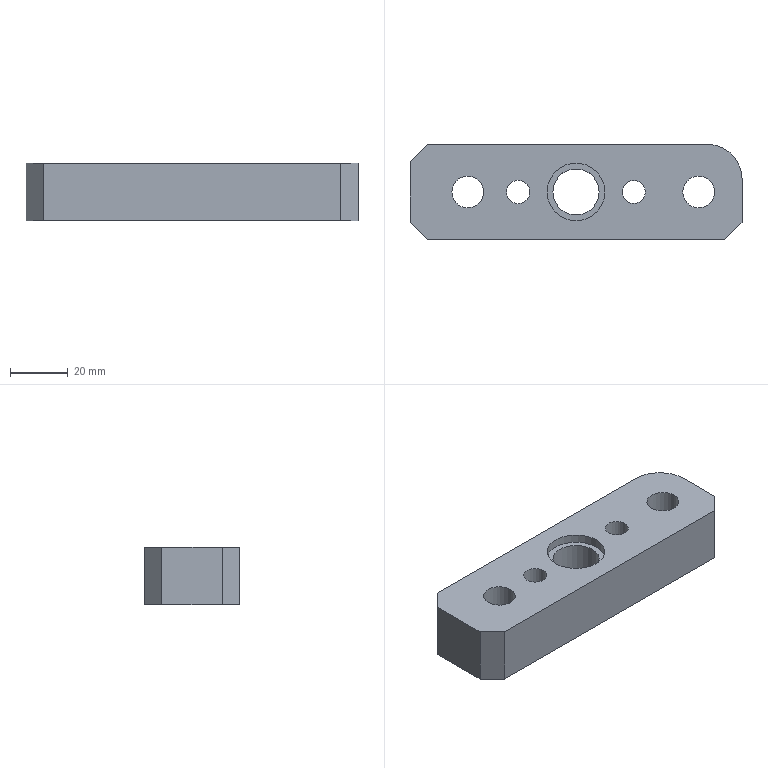Part | STEP file | 103_id3510_x_t | 1 solid | 21 faces | box 115 x 32.999 x 20 mm | volume 61100 mm3 | plane 12 | cylinder 9 | commonest cylinder face diameters 11 x2 17 x2 8 x1 8.1 x1 16 x1 20 x1
STEP:
#1=CARTESIAN_POINT('',(3521.,-0.01549,22.5));
#2=VERTEX_POINT('',#1);
#3=CARTESIAN_POINT('',(3526.5,-0.01549,22.5));
#4=DIRECTION('',(0.,0.,1.));
#5=DIRECTION('',(-1.,0.,0.));
#6=AXIS2_PLACEMENT_3D('',#3,#4,#5);
#7=CIRCLE('',#6,5.5);
#8=EDGE_CURVE('',#2,#2,#7,.T.);
#9=ORIENTED_EDGE('',*,*,#8,.F.);
#10=EDGE_LOOP('',(#9));
#11=FACE_BOUND('',#10,.T.);
#12=CARTESIAN_POINT('',(3601.,-0.01549,22.5));
#13=VERTEX_POINT('',#12);
#14=CARTESIAN_POINT('',(3606.5,-0.01549,22.5));
#15=DIRECTION('',(0.,0.,1.));
#16=DIRECTION('',(-1.,0.,0.));
#17=AXIS2_PLACEMENT_3D('',#14,#15,#16);
#18=CIRCLE('',#17,5.5);
#19=EDGE_CURVE('',#13,#13,#18,.T.);
#20=ORIENTED_EDGE('',*,*,#19,.F.);
#21=EDGE_LOOP('',(#20));
#22=FACE_BOUND('',#21,.T.);
#23=CARTESIAN_POINT('',(3554.,0.,22.5));
#24=VERTEX_POINT('',#23);
#25=CARTESIAN_POINT('',(3564.,0.,22.5));
#26=DIRECTION('',(0.,0.,-1.));
#27=DIRECTION('',(-1.,0.,0.));
#28=AXIS2_PLACEMENT_3D('',#25,#26,#27);
#29=CIRCLE('',#28,10.);
#30=EDGE_CURVE('',#24,#24,#29,.T.);
#31=ORIENTED_EDGE('',*,*,#30,.T.);
#32=EDGE_LOOP('',(#31));
#33=FACE_BOUND('',#32,.T.);
#34=CARTESIAN_POINT('',(3621.5,-10.5,22.5));
#35=VERTEX_POINT('',#34);
#36=CARTESIAN_POINT('',(3621.5,4.5,22.5));
#37=VERTEX_POINT('',#36);
#38=CARTESIAN_POINT('',(3621.5,-172.571,22.5));
#39=DIRECTION('',(0.,1.,0.));
#40=VECTOR('',#39,1.);
#41=LINE('',#38,#40);
#42=EDGE_CURVE('',#35,#37,#41,.T.);
#43=ORIENTED_EDGE('',*,*,#42,.T.);
#44=CARTESIAN_POINT('',(3609.5,16.5,22.5));
#45=VERTEX_POINT('',#44);
#46=CARTESIAN_POINT('',(3609.5,4.5,22.5));
#47=DIRECTION('',(0.,0.,1.));
#48=DIRECTION('',(1.,0.,0.));
#49=AXIS2_PLACEMENT_3D('',#46,#47,#48);
#50=CIRCLE('',#49,12.);
#51=EDGE_CURVE('',#37,#45,#50,.T.);
#52=ORIENTED_EDGE('',*,*,#51,.T.);
#53=CARTESIAN_POINT('',(3512.5,16.5,22.5));
#54=VERTEX_POINT('',#53);
#55=CARTESIAN_POINT('',(4674.5,16.5,22.5));
#56=DIRECTION('',(-1.,0.,0.));
#57=VECTOR('',#56,1.);
#58=LINE('',#55,#57);
#59=EDGE_CURVE('',#45,#54,#58,.T.);
#60=ORIENTED_EDGE('',*,*,#59,.T.);
#61=CARTESIAN_POINT('',(3506.5,10.5,22.5));
#62=VERTEX_POINT('',#61);
#63=CARTESIAN_POINT('',(3998.965,502.965,22.5));
#64=DIRECTION('',(-0.7071,-0.7071,0.));
#65=VECTOR('',#64,1.);
#66=LINE('',#63,#65);
#67=EDGE_CURVE('',#54,#62,#66,.T.);
#68=ORIENTED_EDGE('',*,*,#67,.T.);
#69=CARTESIAN_POINT('',(3506.5,-10.5,22.5));
#70=VERTEX_POINT('',#69);
#71=CARTESIAN_POINT('',(3506.5,-172.571,22.5));
#72=DIRECTION('',(0.,-1.,0.));
#73=VECTOR('',#72,1.);
#74=LINE('',#71,#73);
#75=EDGE_CURVE('',#62,#70,#74,.T.);
#76=ORIENTED_EDGE('',*,*,#75,.T.);
#77=CARTESIAN_POINT('',(3512.5,-16.5,22.5));
#78=VERTEX_POINT('',#77);
#79=CARTESIAN_POINT('',(4171.536,-675.535,22.5));
#80=DIRECTION('',(0.7071,-0.7071,0.));
#81=VECTOR('',#80,1.);
#82=LINE('',#79,#81);
#83=EDGE_CURVE('',#70,#78,#82,.T.);
#84=ORIENTED_EDGE('',*,*,#83,.T.);
#85=CARTESIAN_POINT('',(3615.5,-16.5,22.5));
#86=VERTEX_POINT('',#85);
#87=CARTESIAN_POINT('',(4674.5,-16.5,22.5));
#88=DIRECTION('',(1.,0.,0.));
#89=VECTOR('',#88,1.);
#90=LINE('',#87,#89);
#91=EDGE_CURVE('',#78,#86,#90,.T.);
#92=ORIENTED_EDGE('',*,*,#91,.T.);
#93=CARTESIAN_POINT('',(4066.965,434.965,22.5));
#94=DIRECTION('',(0.7071,0.7071,0.));
#95=VECTOR('',#94,1.);
#96=LINE('',#93,#95);
#97=EDGE_CURVE('',#86,#35,#96,.T.);
#98=ORIENTED_EDGE('',*,*,#97,.T.);
#99=EDGE_LOOP('',(#43,#52,#60,#68,#76,#84,#92,#98));
#100=FACE_BOUND('',#99,.T.);
#101=CARTESIAN_POINT('',(3588.,0.,22.5));
#102=VERTEX_POINT('',#101);
#103=CARTESIAN_POINT('',(3584.,0.,22.5));
#104=DIRECTION('',(0.,0.,1.));
#105=DIRECTION('',(1.,0.,0.));
#106=AXIS2_PLACEMENT_3D('',#103,#104,#105);
#107=CIRCLE('',#106,4.);
#108=EDGE_CURVE('',#102,#102,#107,.T.);
#109=ORIENTED_EDGE('',*,*,#108,.F.);
#110=EDGE_LOOP('',(#109));
#111=FACE_BOUND('',#110,.T.);
#112=CARTESIAN_POINT('',(3548.05,0.,22.5));
#113=VERTEX_POINT('',#112);
#114=CARTESIAN_POINT('',(3544.,0.,22.5));
#115=DIRECTION('',(0.,0.,1.));
#116=DIRECTION('',(1.,0.,0.));
#117=AXIS2_PLACEMENT_3D('',#114,#115,#116);
#118=CIRCLE('',#117,4.05);
#119=EDGE_CURVE('',#113,#113,#118,.T.);
#120=ORIENTED_EDGE('',*,*,#119,.F.);
#121=EDGE_LOOP('',(#120));
#122=FACE_BOUND('',#121,.T.);
#123=CARTESIAN_POINT('',(4674.5,-172.571,22.5));
#124=DIRECTION('',(0.,0.,1.));
#125=DIRECTION('',(-1.,0.,0.));
#126=AXIS2_PLACEMENT_3D('',#123,#124,#125);
#127=PLANE('',#126);
#128=ADVANCED_FACE('',(#11,#22,#33,#100,#111,#122),#127,.T.);
#129=ORIENTED_EDGE('',*,*,#75,.F.);
#130=CARTESIAN_POINT('',(3506.5,10.5,2.5));
#131=VERTEX_POINT('',#130);
#132=CARTESIAN_POINT('',(3506.5,10.5,17.5));
#133=DIRECTION('',(0.,0.,-1.));
#134=VECTOR('',#133,1.);
#135=LINE('',#132,#134);
#136=EDGE_CURVE('',#62,#131,#135,.T.);
#137=ORIENTED_EDGE('',*,*,#136,.T.);
#138=CARTESIAN_POINT('',(3506.5,-10.5,2.5));
#139=VERTEX_POINT('',#138);
#140=CARTESIAN_POINT('',(3506.5,-172.571,2.5));
#141=DIRECTION('',(0.,-1.,0.));
#142=VECTOR('',#141,1.);
#143=LINE('',#140,#142);
#144=EDGE_CURVE('',#131,#139,#143,.T.);
#145=ORIENTED_EDGE('',*,*,#144,.T.);
#146=CARTESIAN_POINT('',(3506.5,-10.5,17.5));
#147=DIRECTION('',(0.,0.,1.));
#148=VECTOR('',#147,1.);
#149=LINE('',#146,#148);
#150=EDGE_CURVE('',#139,#70,#149,.T.);
#151=ORIENTED_EDGE('',*,*,#150,.T.);
#152=EDGE_LOOP('',(#129,#137,#145,#151));
#153=FACE_OUTER_BOUND('',#152,.T.);
#154=CARTESIAN_POINT('',(3506.5,0.,17.5));
#155=DIRECTION('',(-1.,0.,0.));
#156=DIRECTION('',(0.,0.,-1.));
#157=AXIS2_PLACEMENT_3D('',#154,#155,#156);
#158=PLANE('',#157);
#159=ADVANCED_FACE('',(#153),#158,.T.);
#160=CARTESIAN_POINT('',(3621.5,-10.5,2.5));
#161=VERTEX_POINT('',#160);
#162=CARTESIAN_POINT('',(3621.5,4.5,2.5));
#163=VERTEX_POINT('',#162);
#164=CARTESIAN_POINT('',(3621.5,-172.571,2.5));
#165=DIRECTION('',(0.,1.,0.));
#166=VECTOR('',#165,1.);
#167=LINE('',#164,#166);
#168=EDGE_CURVE('',#161,#163,#167,.T.);
#169=ORIENTED_EDGE('',*,*,#168,.T.);
#170=CARTESIAN_POINT('',(3621.5,4.5,22.5));
#171=DIRECTION('',(0.,0.,1.));
#172=VECTOR('',#171,1.);
#173=LINE('',#170,#172);
#174=EDGE_CURVE('',#163,#37,#173,.T.);
#175=ORIENTED_EDGE('',*,*,#174,.T.);
#176=ORIENTED_EDGE('',*,*,#42,.F.);
#177=CARTESIAN_POINT('',(3621.5,-10.5,2.5));
#178=DIRECTION('',(0.,0.,-1.));
#179=VECTOR('',#178,1.);
#180=LINE('',#177,#179);
#181=EDGE_CURVE('',#35,#161,#180,.T.);
#182=ORIENTED_EDGE('',*,*,#181,.T.);
#183=EDGE_LOOP('',(#169,#175,#176,#182));
#184=FACE_OUTER_BOUND('',#183,.T.);
#185=CARTESIAN_POINT('',(3621.5,-172.571,2.5));
#186=DIRECTION('',(-1.,0.,0.));
#187=DIRECTION('',(0.,-1.,0.));
#188=AXIS2_PLACEMENT_3D('',#185,#186,#187);
#189=PLANE('',#188);
#190=ADVANCED_FACE('',(#184),#189,.F.);
#191=CARTESIAN_POINT('',(3580.,0.,2.5));
#192=VERTEX_POINT('',#191);
#193=CARTESIAN_POINT('',(3584.,0.,2.5));
#194=DIRECTION('',(0.,0.,-1.));
#195=DIRECTION('',(-1.,0.,0.));
#196=AXIS2_PLACEMENT_3D('',#193,#194,#195);
#197=CIRCLE('',#196,4.);
#198=EDGE_CURVE('',#192,#192,#197,.T.);
#199=ORIENTED_EDGE('',*,*,#198,.F.);
#200=EDGE_LOOP('',(#199));
#201=FACE_BOUND('',#200,.T.);
#202=CARTESIAN_POINT('',(3539.95,0.,2.5));
#203=VERTEX_POINT('',#202);
#204=CARTESIAN_POINT('',(3544.,0.,2.5));
#205=DIRECTION('',(0.,0.,1.));
#206=DIRECTION('',(-1.,0.,0.));
#207=AXIS2_PLACEMENT_3D('',#204,#205,#206);
#208=CIRCLE('',#207,4.05);
#209=EDGE_CURVE('',#203,#203,#208,.T.);
#210=ORIENTED_EDGE('',*,*,#209,.T.);
#211=EDGE_LOOP('',(#210));
#212=FACE_BOUND('',#211,.T.);
#213=CARTESIAN_POINT('',(3556.,0.,2.5));
#214=VERTEX_POINT('',#213);
#215=CARTESIAN_POINT('',(3564.,0.,2.5));
#216=DIRECTION('',(0.,0.,1.));
#217=DIRECTION('',(-1.,0.,0.));
#218=AXIS2_PLACEMENT_3D('',#215,#216,#217);
#219=CIRCLE('',#218,8.);
#220=EDGE_CURVE('',#214,#214,#219,.T.);
#221=ORIENTED_EDGE('',*,*,#220,.T.);
#222=EDGE_LOOP('',(#221));
#223=FACE_BOUND('',#222,.T.);
#224=CARTESIAN_POINT('',(3518.,-0.01549,2.5));
#225=VERTEX_POINT('',#224);
#226=CARTESIAN_POINT('',(3526.5,-0.01549,2.5));
#227=DIRECTION('',(0.,0.,1.));
#228=DIRECTION('',(-1.,0.,0.));
#229=AXIS2_PLACEMENT_3D('',#226,#227,#228);
#230=CIRCLE('',#229,8.5);
#231=EDGE_CURVE('',#225,#225,#230,.T.);
#232=ORIENTED_EDGE('',*,*,#231,.T.);
#233=EDGE_LOOP('',(#232));
#234=FACE_BOUND('',#233,.T.);
#235=CARTESIAN_POINT('',(3598.,-0.01549,2.5));
#236=VERTEX_POINT('',#235);
#237=CARTESIAN_POINT('',(3606.5,-0.01549,2.5));
#238=DIRECTION('',(0.,0.,1.));
#239=DIRECTION('',(-1.,0.,0.));
#240=AXIS2_PLACEMENT_3D('',#237,#238,#239);
#241=CIRCLE('',#240,8.5);
#242=EDGE_CURVE('',#236,#236,#241,.T.);
#243=ORIENTED_EDGE('',*,*,#242,.T.);
#244=EDGE_LOOP('',(#243));
#245=FACE_BOUND('',#244,.T.);
#246=CARTESIAN_POINT('',(3609.5,16.5,2.5));
#247=VERTEX_POINT('',#246);
#248=CARTESIAN_POINT('',(3512.5,16.5,2.5));
#249=VERTEX_POINT('',#248);
#250=CARTESIAN_POINT('',(3486.688,16.5,2.5));
#251=DIRECTION('',(-1.,0.,0.));
#252=VECTOR('',#251,1.);
#253=LINE('',#250,#252);
#254=EDGE_CURVE('',#247,#249,#253,.T.);
#255=ORIENTED_EDGE('',*,*,#254,.F.);
#256=CARTESIAN_POINT('',(3609.5,4.5,2.5));
#257=DIRECTION('',(0.,0.,-1.));
#258=DIRECTION('',(1.,0.,0.));
#259=AXIS2_PLACEMENT_3D('',#256,#257,#258);
#260=CIRCLE('',#259,12.);
#261=EDGE_CURVE('',#247,#163,#260,.T.);
#262=ORIENTED_EDGE('',*,*,#261,.T.);
#263=ORIENTED_EDGE('',*,*,#168,.F.);
#264=CARTESIAN_POINT('',(3615.5,-16.5,2.5));
#265=VERTEX_POINT('',#264);
#266=CARTESIAN_POINT('',(3621.5,-10.5,2.5));
#267=DIRECTION('',(-0.7071,-0.7071,0.));
#268=VECTOR('',#267,1.);
#269=LINE('',#266,#268);
#270=EDGE_CURVE('',#161,#265,#269,.T.);
#271=ORIENTED_EDGE('',*,*,#270,.T.);
#272=CARTESIAN_POINT('',(3512.5,-16.5,2.5));
#273=VERTEX_POINT('',#272);
#274=CARTESIAN_POINT('',(3486.688,-16.5,2.5));
#275=DIRECTION('',(1.,0.,0.));
#276=VECTOR('',#275,1.);
#277=LINE('',#274,#276);
#278=EDGE_CURVE('',#273,#265,#277,.T.);
#279=ORIENTED_EDGE('',*,*,#278,.F.);
#280=CARTESIAN_POINT('',(3512.5,-16.5,2.5));
#281=DIRECTION('',(-0.7071,0.7071,0.));
#282=VECTOR('',#281,1.);
#283=LINE('',#280,#282);
#284=EDGE_CURVE('',#273,#139,#283,.T.);
#285=ORIENTED_EDGE('',*,*,#284,.T.);
#286=ORIENTED_EDGE('',*,*,#144,.F.);
#287=CARTESIAN_POINT('',(3512.5,16.5,2.5));
#288=DIRECTION('',(0.7071,0.7071,0.));
#289=VECTOR('',#288,1.);
#290=LINE('',#287,#289);
#291=EDGE_CURVE('',#131,#249,#290,.T.);
#292=ORIENTED_EDGE('',*,*,#291,.T.);
#293=EDGE_LOOP('',(#255,#262,#263,#271,#279,#285,#286,#292));
#294=FACE_BOUND('',#293,.T.);
#295=CARTESIAN_POINT('',(4674.5,-172.571,2.5));
#296=DIRECTION('',(0.,0.,1.));
#297=DIRECTION('',(-1.,0.,0.));
#298=AXIS2_PLACEMENT_3D('',#295,#296,#297);
#299=PLANE('',#298);
#300=ADVANCED_FACE('',(#201,#212,#223,#234,#245,#294),#299,.F.);
#301=CARTESIAN_POINT('',(3598.,-0.01549,13.5));
#302=VERTEX_POINT('',#301);
#303=CARTESIAN_POINT('',(3606.5,-0.01549,13.5));
#304=DIRECTION('',(0.,0.,-1.));
#305=DIRECTION('',(-1.,0.,0.));
#306=AXIS2_PLACEMENT_3D('',#303,#304,#305);
#307=CIRCLE('',#306,8.5);
#308=EDGE_CURVE('',#302,#302,#307,.T.);
#309=ORIENTED_EDGE('',*,*,#308,.F.);
#310=EDGE_LOOP('',(#309));
#311=FACE_BOUND('',#310,.T.);
#312=ORIENTED_EDGE('',*,*,#242,.F.);
#313=EDGE_LOOP('',(#312));
#314=FACE_BOUND('',#313,.T.);
#315=CARTESIAN_POINT('',(3606.5,-0.01549,-35.5));
#316=DIRECTION('',(0.,0.,1.));
#317=DIRECTION('',(-1.,0.,0.));
#318=AXIS2_PLACEMENT_3D('',#315,#316,#317);
#319=CYLINDRICAL_SURFACE('',#318,8.5);
#320=ADVANCED_FACE('',(#311,#314),#319,.F.);
#321=CARTESIAN_POINT('',(3601.,-0.01549,13.5));
#322=VERTEX_POINT('',#321);
#323=CARTESIAN_POINT('',(3606.5,-0.01549,13.5));
#324=DIRECTION('',(0.,0.,-1.));
#325=DIRECTION('',(-1.,0.,0.));
#326=AXIS2_PLACEMENT_3D('',#323,#324,#325);
#327=CIRCLE('',#326,5.5);
#328=EDGE_CURVE('',#322,#322,#327,.T.);
#329=ORIENTED_EDGE('',*,*,#328,.F.);
#330=EDGE_LOOP('',(#329));
#331=FACE_BOUND('',#330,.T.);
#332=ORIENTED_EDGE('',*,*,#308,.T.);
#333=EDGE_LOOP('',(#332));
#334=FACE_BOUND('',#333,.T.);
#335=CARTESIAN_POINT('',(3606.5,-0.01549,13.5));
#336=DIRECTION('',(0.,0.,1.));
#337=DIRECTION('',(-1.,0.,0.));
#338=AXIS2_PLACEMENT_3D('',#335,#336,#337);
#339=PLANE('',#338);
#340=ADVANCED_FACE('',(#331,#334),#339,.F.);
#341=ORIENTED_EDGE('',*,*,#19,.T.);
#342=EDGE_LOOP('',(#341));
#343=FACE_BOUND('',#342,.T.);
#344=ORIENTED_EDGE('',*,*,#328,.T.);
#345=EDGE_LOOP('',(#344));
#346=FACE_BOUND('',#345,.T.);
#347=CARTESIAN_POINT('',(3606.5,-0.01549,14.5));
#348=DIRECTION('',(0.,0.,1.));
#349=DIRECTION('',(-1.,0.,0.));
#350=AXIS2_PLACEMENT_3D('',#347,#348,#349);
#351=CYLINDRICAL_SURFACE('',#350,5.5);
#352=ADVANCED_FACE('',(#343,#346),#351,.F.);
#353=CARTESIAN_POINT('',(3518.,-0.01549,13.5));
#354=VERTEX_POINT('',#353);
#355=CARTESIAN_POINT('',(3526.5,-0.01549,13.5));
#356=DIRECTION('',(0.,0.,1.));
#357=DIRECTION('',(-1.,0.,0.));
#358=AXIS2_PLACEMENT_3D('',#355,#356,#357);
#359=CIRCLE('',#358,8.5);
#360=EDGE_CURVE('',#354,#354,#359,.T.);
#361=ORIENTED_EDGE('',*,*,#360,.T.);
#362=EDGE_LOOP('',(#361));
#363=FACE_BOUND('',#362,.T.);
#364=ORIENTED_EDGE('',*,*,#231,.F.);
#365=EDGE_LOOP('',(#364));
#366=FACE_BOUND('',#365,.T.);
#367=CARTESIAN_POINT('',(3526.5,-0.01549,-35.5));
#368=DIRECTION('',(0.,0.,1.));
#369=DIRECTION('',(1.,0.,0.));
#370=AXIS2_PLACEMENT_3D('',#367,#368,#369);
#371=CYLINDRICAL_SURFACE('',#370,8.5);
#372=ADVANCED_FACE('',(#363,#366),#371,.F.);
#373=CARTESIAN_POINT('',(3521.,-0.01549,13.5));
#374=VERTEX_POINT('',#373);
#375=CARTESIAN_POINT('',(3526.5,-0.01549,13.5));
#376=DIRECTION('',(0.,0.,1.));
#377=DIRECTION('',(-1.,0.,0.));
#378=AXIS2_PLACEMENT_3D('',#375,#376,#377);
#379=CIRCLE('',#378,5.5);
#380=EDGE_CURVE('',#374,#374,#379,.T.);
#381=ORIENTED_EDGE('',*,*,#380,.T.);
#382=EDGE_LOOP('',(#381));
#383=FACE_BOUND('',#382,.T.);
#384=ORIENTED_EDGE('',*,*,#360,.F.);
#385=EDGE_LOOP('',(#384));
#386=FACE_BOUND('',#385,.T.);
#387=CARTESIAN_POINT('',(3526.5,-0.01549,13.5));
#388=DIRECTION('',(0.,0.,1.));
#389=DIRECTION('',(1.,0.,0.));
#390=AXIS2_PLACEMENT_3D('',#387,#388,#389);
#391=PLANE('',#390);
#392=ADVANCED_FACE('',(#383,#386),#391,.F.);
#393=ORIENTED_EDGE('',*,*,#8,.T.);
#394=EDGE_LOOP('',(#393));
#395=FACE_BOUND('',#394,.T.);
#396=ORIENTED_EDGE('',*,*,#380,.F.);
#397=EDGE_LOOP('',(#396));
#398=FACE_BOUND('',#397,.T.);
#399=CARTESIAN_POINT('',(3526.5,-0.01549,14.5));
#400=DIRECTION('',(0.,0.,1.));
#401=DIRECTION('',(1.,0.,0.));
#402=AXIS2_PLACEMENT_3D('',#399,#400,#401);
#403=CYLINDRICAL_SURFACE('',#402,5.5);
#404=ADVANCED_FACE('',(#395,#398),#403,.F.);
#405=ORIENTED_EDGE('',*,*,#209,.F.);
#406=EDGE_LOOP('',(#405));
#407=FACE_BOUND('',#406,.T.);
#408=ORIENTED_EDGE('',*,*,#119,.T.);
#409=EDGE_LOOP('',(#408));
#410=FACE_BOUND('',#409,.T.);
#411=CARTESIAN_POINT('',(3544.,0.,-40.259));
#412=DIRECTION('',(0.,0.,1.));
#413=DIRECTION('',(0.,-1.,0.));
#414=AXIS2_PLACEMENT_3D('',#411,#412,#413);
#415=CYLINDRICAL_SURFACE('',#414,4.05);
#416=ADVANCED_FACE('',(#407,#410),#415,.F.);
#417=CARTESIAN_POINT('',(3556.,0.,19.5));
#418=VERTEX_POINT('',#417);
#419=CARTESIAN_POINT('',(3564.,0.,19.5));
#420=DIRECTION('',(0.,0.,1.));
#421=DIRECTION('',(-1.,0.,0.));
#422=AXIS2_PLACEMENT_3D('',#419,#420,#421);
#423=CIRCLE('',#422,8.);
#424=EDGE_CURVE('',#418,#418,#423,.T.);
#425=ORIENTED_EDGE('',*,*,#424,.T.);
#426=EDGE_LOOP('',(#425));
#427=FACE_BOUND('',#426,.T.);
#428=ORIENTED_EDGE('',*,*,#220,.F.);
#429=EDGE_LOOP('',(#428));
#430=FACE_BOUND('',#429,.T.);
#431=CARTESIAN_POINT('',(3564.,0.,25.));
#432=DIRECTION('',(0.,0.,-1.));
#433=DIRECTION('',(1.,0.,0.));
#434=AXIS2_PLACEMENT_3D('',#431,#432,#433);
#435=CYLINDRICAL_SURFACE('',#434,8.);
#436=ADVANCED_FACE('',(#427,#430),#435,.F.);
#437=CARTESIAN_POINT('',(3554.,0.,19.5));
#438=VERTEX_POINT('',#437);
#439=CARTESIAN_POINT('',(3564.,0.,19.5));
#440=DIRECTION('',(0.,0.,1.));
#441=DIRECTION('',(-1.,0.,0.));
#442=AXIS2_PLACEMENT_3D('',#439,#440,#441);
#443=CIRCLE('',#442,10.);
#444=EDGE_CURVE('',#438,#438,#443,.T.);
#445=ORIENTED_EDGE('',*,*,#444,.T.);
#446=EDGE_LOOP('',(#445));
#447=FACE_BOUND('',#446,.T.);
#448=ORIENTED_EDGE('',*,*,#424,.F.);
#449=EDGE_LOOP('',(#448));
#450=FACE_BOUND('',#449,.T.);
#451=CARTESIAN_POINT('',(3564.,0.,19.5));
#452=DIRECTION('',(0.,0.,-1.));
#453=DIRECTION('',(1.,0.,0.));
#454=AXIS2_PLACEMENT_3D('',#451,#452,#453);
#455=PLANE('',#454);
#456=ADVANCED_FACE('',(#447,#450),#455,.F.);
#457=ORIENTED_EDGE('',*,*,#30,.F.);
#458=EDGE_LOOP('',(#457));
#459=FACE_BOUND('',#458,.T.);
#460=ORIENTED_EDGE('',*,*,#444,.F.);
#461=EDGE_LOOP('',(#460));
#462=FACE_BOUND('',#461,.T.);
#463=CARTESIAN_POINT('',(3564.,0.,17.5));
#464=DIRECTION('',(0.,0.,-1.));
#465=DIRECTION('',(1.,0.,0.));
#466=AXIS2_PLACEMENT_3D('',#463,#464,#465);
#467=CYLINDRICAL_SURFACE('',#466,10.);
#468=ADVANCED_FACE('',(#459,#462),#467,.F.);
#469=ORIENTED_EDGE('',*,*,#108,.T.);
#470=EDGE_LOOP('',(#469));
#471=FACE_BOUND('',#470,.T.);
#472=ORIENTED_EDGE('',*,*,#198,.T.);
#473=EDGE_LOOP('',(#472));
#474=FACE_BOUND('',#473,.T.);
#475=CARTESIAN_POINT('',(3584.,0.,-40.259));
#476=DIRECTION('',(0.,0.,1.));
#477=DIRECTION('',(0.,1.,0.));
#478=AXIS2_PLACEMENT_3D('',#475,#476,#477);
#479=CYLINDRICAL_SURFACE('',#478,4.);
#480=ADVANCED_FACE('',(#471,#474),#479,.F.);
#481=ORIENTED_EDGE('',*,*,#278,.T.);
#482=CARTESIAN_POINT('',(3615.5,-16.5,22.5));
#483=DIRECTION('',(0.,0.,1.));
#484=VECTOR('',#483,1.);
#485=LINE('',#482,#484);
#486=EDGE_CURVE('',#265,#86,#485,.T.);
#487=ORIENTED_EDGE('',*,*,#486,.T.);
#488=ORIENTED_EDGE('',*,*,#91,.F.);
#489=CARTESIAN_POINT('',(3512.5,-16.5,3.46));
#490=DIRECTION('',(0.,0.,-1.));
#491=VECTOR('',#490,1.);
#492=LINE('',#489,#491);
#493=EDGE_CURVE('',#78,#273,#492,.T.);
#494=ORIENTED_EDGE('',*,*,#493,.T.);
#495=EDGE_LOOP('',(#481,#487,#488,#494));
#496=FACE_OUTER_BOUND('',#495,.T.);
#497=CARTESIAN_POINT('',(3486.688,-16.5,3.46));
#498=DIRECTION('',(0.,-1.,0.));
#499=DIRECTION('',(0.,0.,1.));
#500=AXIS2_PLACEMENT_3D('',#497,#498,#499);
#501=PLANE('',#500);
#502=ADVANCED_FACE('',(#496),#501,.T.);
#503=ORIENTED_EDGE('',*,*,#59,.F.);
#504=CARTESIAN_POINT('',(3609.5,16.5,2.5));
#505=DIRECTION('',(0.,0.,-1.));
#506=VECTOR('',#505,1.);
#507=LINE('',#504,#506);
#508=EDGE_CURVE('',#45,#247,#507,.T.);
#509=ORIENTED_EDGE('',*,*,#508,.T.);
#510=ORIENTED_EDGE('',*,*,#254,.T.);
#511=CARTESIAN_POINT('',(3512.5,16.5,3.46));
#512=DIRECTION('',(0.,0.,1.));
#513=VECTOR('',#512,1.);
#514=LINE('',#511,#513);
#515=EDGE_CURVE('',#249,#54,#514,.T.);
#516=ORIENTED_EDGE('',*,*,#515,.T.);
#517=EDGE_LOOP('',(#503,#509,#510,#516));
#518=FACE_OUTER_BOUND('',#517,.T.);
#519=CARTESIAN_POINT('',(3486.688,16.5,3.46));
#520=DIRECTION('',(0.,1.,0.));
#521=DIRECTION('',(0.,0.,-1.));
#522=AXIS2_PLACEMENT_3D('',#519,#520,#521);
#523=PLANE('',#522);
#524=ADVANCED_FACE('',(#518),#523,.T.);
#525=ORIENTED_EDGE('',*,*,#291,.F.);
#526=ORIENTED_EDGE('',*,*,#136,.F.);
#527=ORIENTED_EDGE('',*,*,#67,.F.);
#528=ORIENTED_EDGE('',*,*,#515,.F.);
#529=EDGE_LOOP('',(#525,#526,#527,#528));
#530=FACE_OUTER_BOUND('',#529,.T.);
#531=CARTESIAN_POINT('',(3512.5,16.5,3.46));
#532=DIRECTION('',(0.7071,-0.7071,0.));
#533=DIRECTION('',(0.,0.,-1.));
#534=AXIS2_PLACEMENT_3D('',#531,#532,#533);
#535=PLANE('',#534);
#536=ADVANCED_FACE('',(#530),#535,.F.);
#537=ORIENTED_EDGE('',*,*,#97,.F.);
#538=ORIENTED_EDGE('',*,*,#486,.F.);
#539=ORIENTED_EDGE('',*,*,#270,.F.);
#540=ORIENTED_EDGE('',*,*,#181,.F.);
#541=EDGE_LOOP('',(#537,#538,#539,#540));
#542=FACE_OUTER_BOUND('',#541,.T.);
#543=CARTESIAN_POINT('',(3621.5,-10.5,2.5));
#544=DIRECTION('',(0.7071,-0.7071,0.));
#545=DIRECTION('',(0.,0.,-1.));
#546=AXIS2_PLACEMENT_3D('',#543,#544,#545);
#547=PLANE('',#546);
#548=ADVANCED_FACE('',(#542),#547,.T.);
#549=ORIENTED_EDGE('',*,*,#83,.F.);
#550=ORIENTED_EDGE('',*,*,#150,.F.);
#551=ORIENTED_EDGE('',*,*,#284,.F.);
#552=ORIENTED_EDGE('',*,*,#493,.F.);
#553=EDGE_LOOP('',(#549,#550,#551,#552));
#554=FACE_OUTER_BOUND('',#553,.T.);
#555=CARTESIAN_POINT('',(3512.5,-16.5,3.46));
#556=DIRECTION('',(0.7071,0.7071,0.));
#557=DIRECTION('',(0.,0.,1.));
#558=AXIS2_PLACEMENT_3D('',#555,#556,#557);
#559=PLANE('',#558);
#560=ADVANCED_FACE('',(#554),#559,.F.);
#561=ORIENTED_EDGE('',*,*,#51,.F.);
#562=ORIENTED_EDGE('',*,*,#174,.F.);
#563=ORIENTED_EDGE('',*,*,#261,.F.);
#564=ORIENTED_EDGE('',*,*,#508,.F.);
#565=EDGE_LOOP('',(#561,#562,#563,#564));
#566=FACE_OUTER_BOUND('',#565,.T.);
#567=CARTESIAN_POINT('',(3609.5,4.5,3.46));
#568=DIRECTION('',(0.,0.,1.));
#569=DIRECTION('',(-1.,0.,0.));
#570=AXIS2_PLACEMENT_3D('',#567,#568,#569);
#571=CYLINDRICAL_SURFACE('',#570,12.);
#572=ADVANCED_FACE('',(#566),#571,.T.);
#573=CLOSED_SHELL('',(#128,#159,#190,#300,#320,#340,#352,#372,#392,#404,#416,#436,#456,#468,#480,#502,#524,#536,#548,#560,#572));
#574=MANIFOLD_SOLID_BREP('',#573);
#575=(LENGTH_UNIT()NAMED_UNIT(*)SI_UNIT(.MILLI.,.METRE.));
#576=UNCERTAINTY_MEASURE_WITH_UNIT(LENGTH_MEASURE(0.00002),#575,'','');
#577=(NAMED_UNIT(*)PLANE_ANGLE_UNIT()SI_UNIT($,.RADIAN.));
#578=PLANE_ANGLE_MEASURE_WITH_UNIT(PLANE_ANGLE_MEASURE(0.01745),#577);
#579=DIMENSIONAL_EXPONENTS(0.,0.,0.,0.,0.,0.,0.);
#580=(CONVERSION_BASED_UNIT('DEGREE',#578)NAMED_UNIT(#579)PLANE_ANGLE_UNIT());
#581=(NAMED_UNIT(*)SI_UNIT($,.STERADIAN.)SOLID_ANGLE_UNIT());
#582=(GEOMETRIC_REPRESENTATION_CONTEXT(3)GLOBAL_UNCERTAINTY_ASSIGNED_CONTEXT((#576))GLOBAL_UNIT_ASSIGNED_CONTEXT((#575,#580,#581))REPRESENTATION_CONTEXT('',''));
#583=ADVANCED_BREP_SHAPE_REPRESENTATION('',(#574),#582);